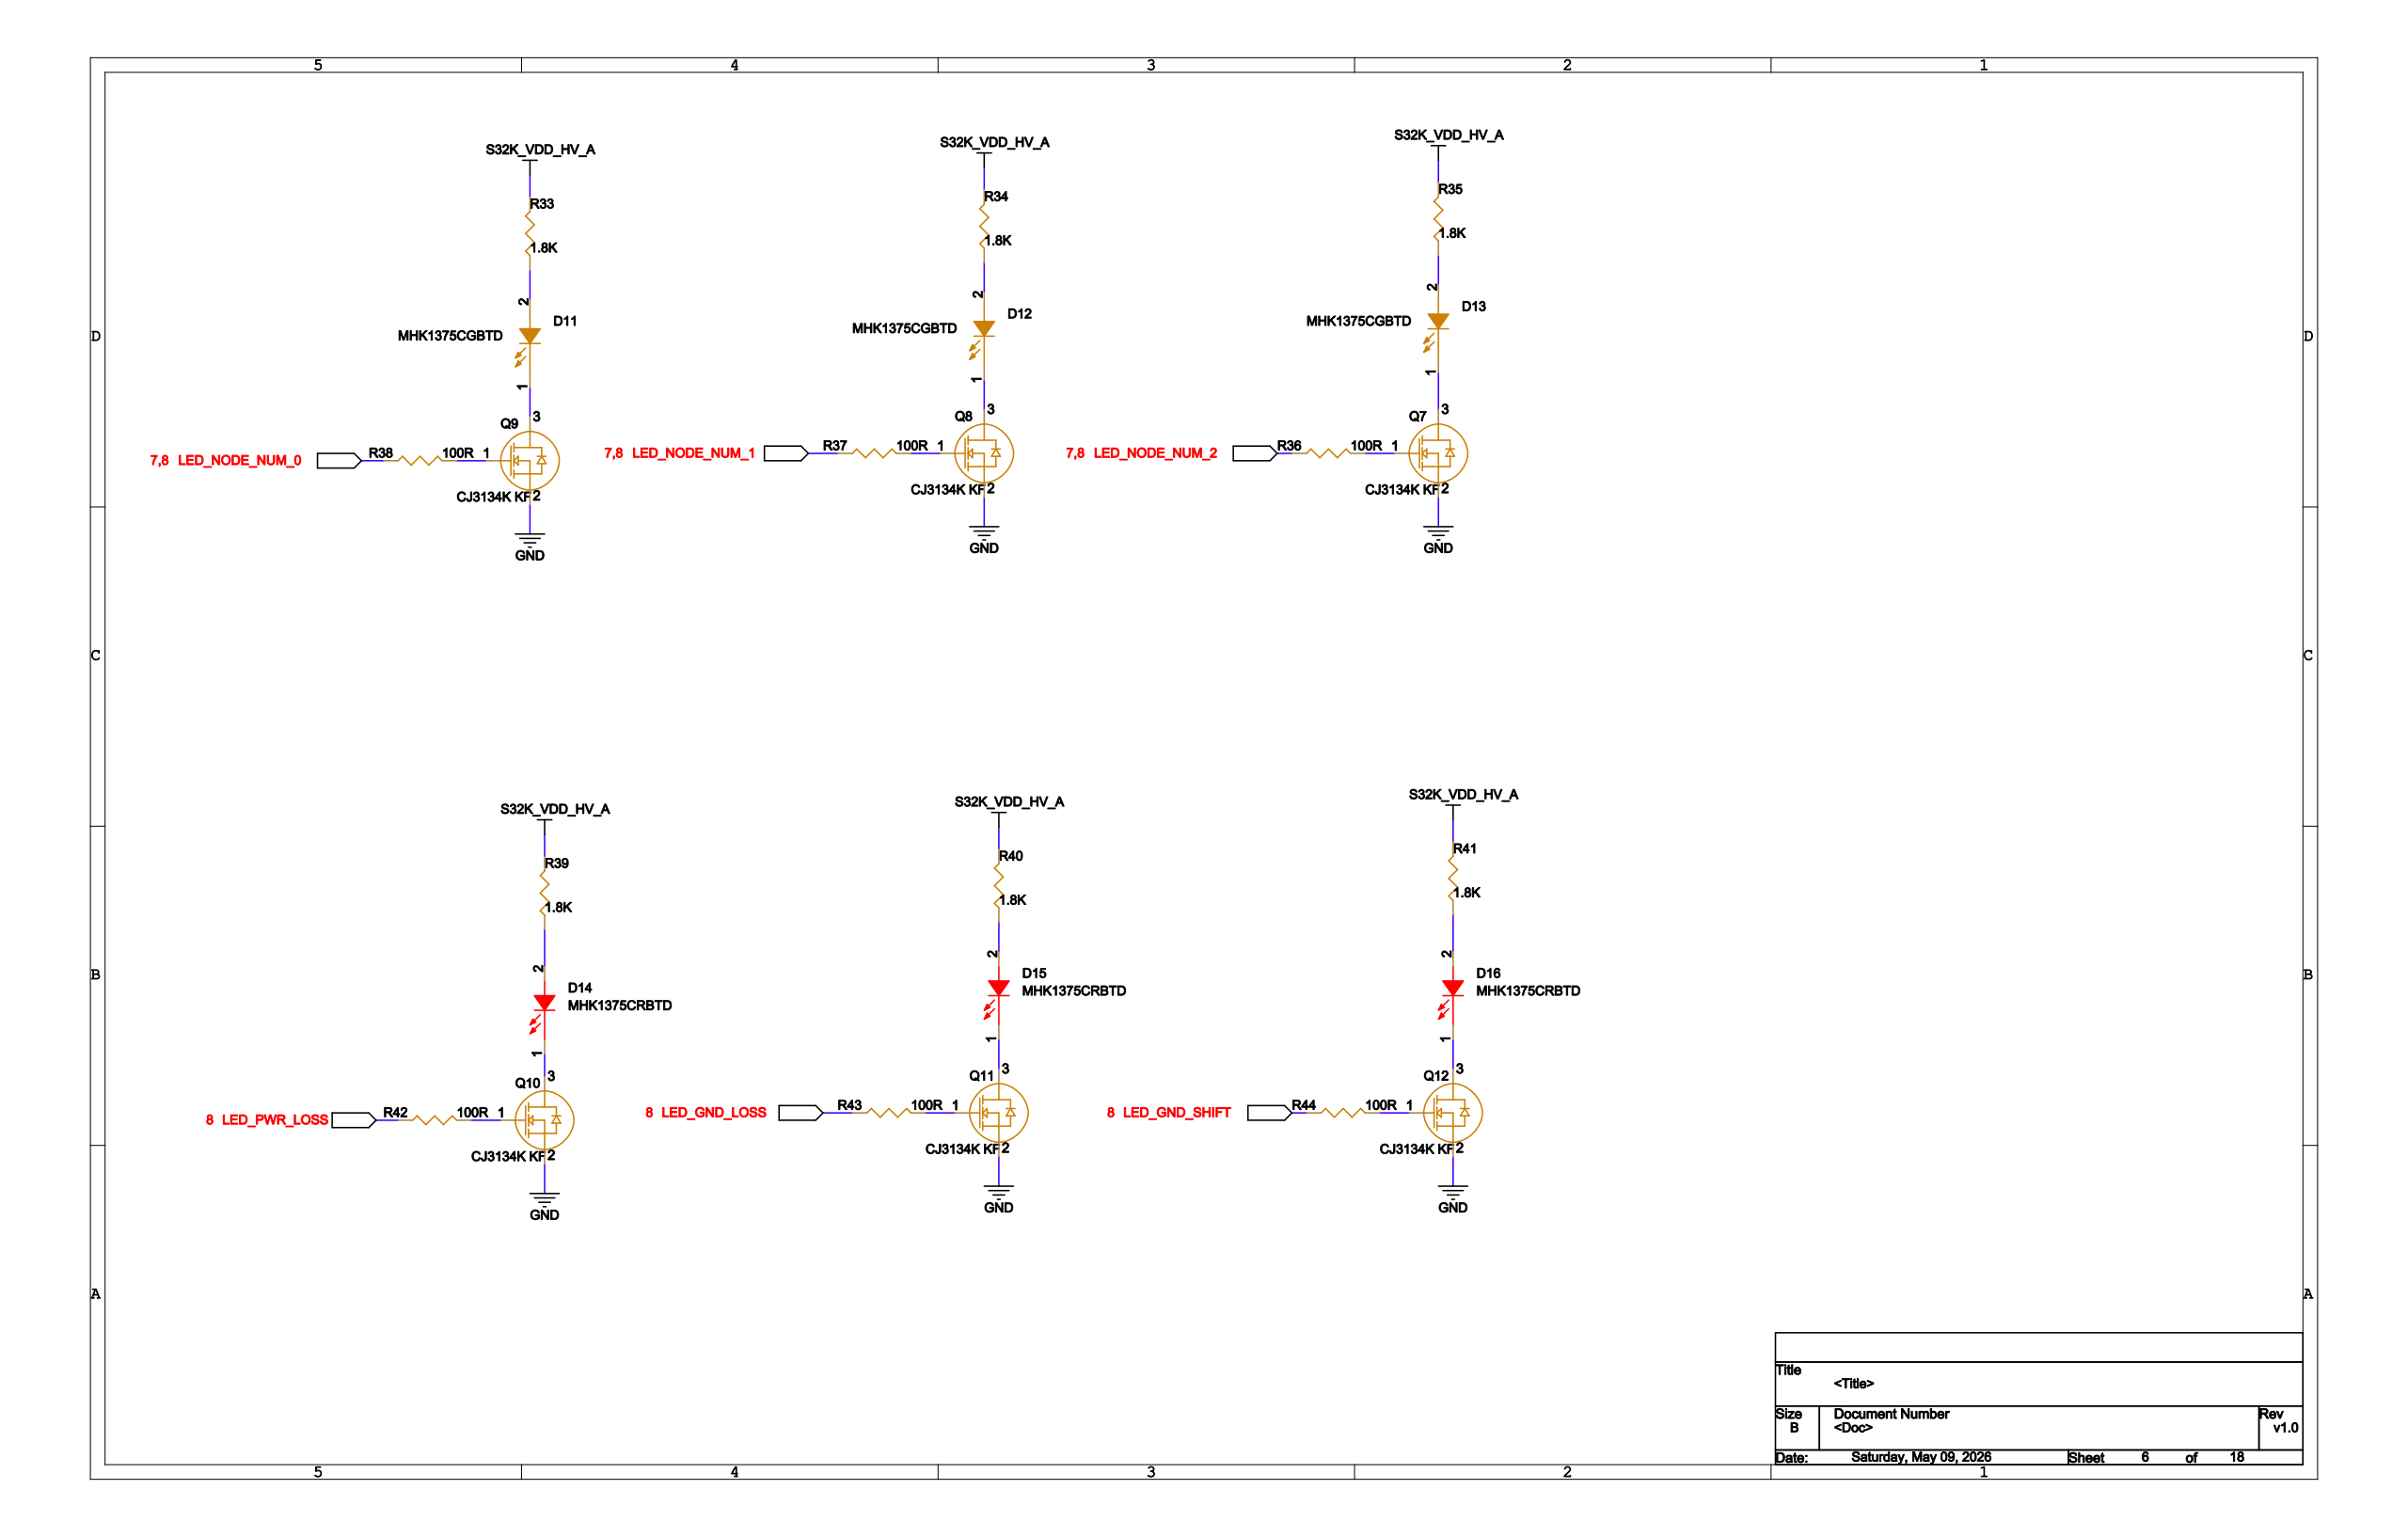Circuit board | Cadence Allegro | 330 parts | 215 nets | one sheet of the schematic
Parts on this sheet (reference | value | footprint):
D11 | MHK1375CGBTD | LED-TH_MHK1375CRBTD
D12 | MHK1375CGBTD | LED-TH_MHK1375CRBTD
D13 | MHK1375CGBTD | LED-TH_MHK1375CRBTD
D14 | MHK1375CRBTD | LED-TH_MHK1375CRBTD
D15 | MHK1375CRBTD | LED-TH_MHK1375CRBTD
D16 | MHK1375CRBTD | LED-TH_MHK1375CRBTD
Q7 | CJ3134K KF | SOT-723
Q8 | CJ3134K KF | SOT-723
Q9 | CJ3134K KF | SOT-723
Q10 | CJ3134K KF | SOT-723
Q11 | CJ3134K KF | SOT-723
Q12 | CJ3134K KF | SOT-723
R33 | 1.8K | 0402
R34 | 1.8K | 0402
R35 | 1.8K | 0402
R36 | 100R | 0402
R37 | 100R | 0402
R38 | 100R | 0402
R39 | 1.8K | 0402
R40 | 1.8K | 0402
R41 | 1.8K | 0402
R42 | 100R | 0402
R43 | 100R | 0402
R44 | 100R | 0402
Nets of these parts (net: part-pin ...):
GND: Q7-2 Q8-2 Q9-2 Q10-2 Q11-2 Q12-2
S32K_VDD_HV_A: R33-2 R34-2 R35-2 R39-2 R40-2 R41-2
N16857287: D11-1 Q9-3
N16781463: D11-2 R33-1
N16959625: D12-1 Q8-3
N16781465: D12-2 R34-1
N16857431: D13-1 Q7-3
N16857128: D13-2 R35-1
N16959440: D14-1 Q10-3
N16959396: D14-2 R39-1
N16959436: D15-1 Q11-3
N16959398: D15-2 R40-1
N16959438: D16-1 Q12-3
N16959394: D16-2 R41-1
N16959510: Q10-1 R42-2
N16959514: Q11-1 R43-2
N16959518: Q12-1 R44-2
N16857457: Q7-1 R36-2
N16857362: Q8-1 R37-2
N16857208: Q9-1 R38-2
LED_NODE_NUM_0: R38-1
LED_NODE_NUM_1: R37-1
LED_NODE_NUM_2: R36-1
LED_PWR_LOSS: R42-1
LED_GND_LOSS: R43-1
LED_GND_SHIFT: R44-1